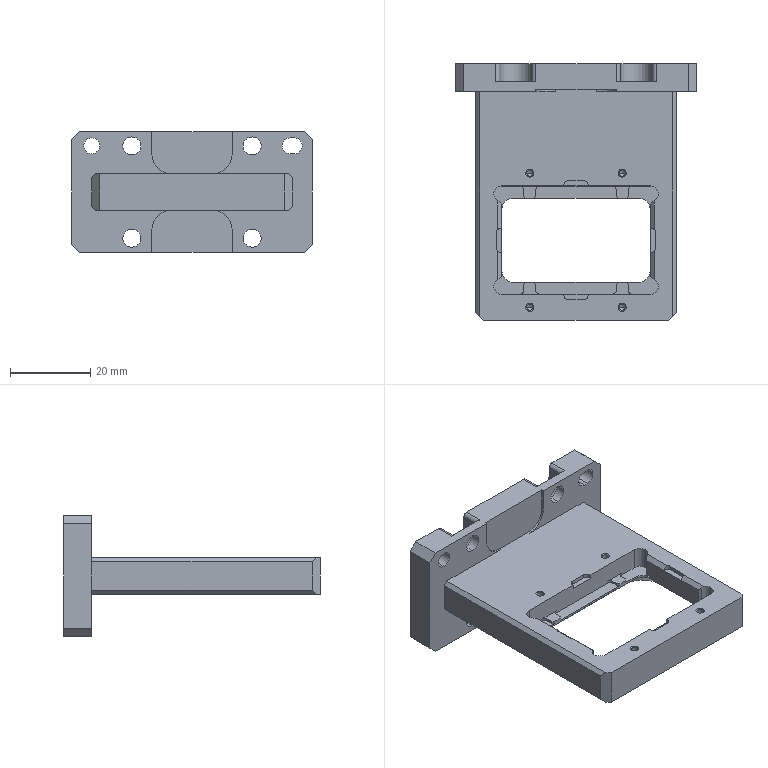NC program | NX | posted with a generic post | part box 60 x 64 x 30 mm
Lines 1 to 592 of 2202:
N10 G17 G21 G94 G90
(ZLEVEL_PROFILE_1 , TOOL : D6)
N12 T06 M6
N14 G54
N16 G17 G0 G90 X20.505 Y-18.6 B0. C0. S9500 M3
N18 G43 Z30. H6
N20 Z0.54
N22 G94 G1 Z-0.46 F1650.
N24 X20.356 Y-18.317
N26 G3 X19.848 Y-17.997 R0.6
N28 G2 X16. Y-14. R4.
N30 G1 Y-11.48
N32 G3 X15. Y-10.48 R1.
N34 X14. Y-11.48 R1.
N36 G1 Y-14.
N38 G2 X10.159 Y-17.997 R4.
N40 G3 X9.652 Y-18.317 R0.6
N42 G1 X9.503 Y-18.6
N44 Z0.54
N46 G0 X20.507 Z0.08
N48 G1 Z-0.92
N50 X20.356 Y-18.316
N52 G3 X19.848 Y-17.997 R0.6
N54 G1 X19.823 Y-17.996
N56 G2 X16. Y-14. R4.
N58 G1 Y-11.48
N60 G3 X15. Y-10.48 R1.
N62 X14. Y-11.48 R1.
N64 G1 Y-14.
N66 G2 X10.159 Y-17.996 R4.
N68 G3 X9.646 Y-18.308 R0.6
N70 G1 X9.487 Y-18.6
N72 Z0.08
N74 G0 X20.483 Z-0.38
N76 G1 Z-1.38
N78 X20.345 Y-18.326
N80 G3 X19.843 Y-17.997 R0.6
N82 G1 X19.823 Y-17.996
N84 G2 X16. Y-14. R4.
N86 G1 Y-11.48
N88 G3 X15. Y-10.48 R1.
N90 X14. Y-11.48 R1.
N92 G1 Y-14.
N94 G2 X10.159 Y-17.997 R4.
N96 G3 X9.649 Y-18.312 R0.6
N98 G1 X9.494 Y-18.6
N100 Z-0.38
N102 G0 X20.467 Z-0.84
N104 G1 Z-1.84
N106 X20.339 Y-18.335
N108 G3 X19.843 Y-17.998 R0.6
N110 G1 X19.823 Y-17.996
N112 G2 X16. Y-14. R4.
N114 G1 Y-11.48
N116 G3 X15. Y-10.48 R1.
N118 X14. Y-11.48 R1.
N120 G1 Y-14.
N122 G2 X10.159 Y-17.997 R4.
N124 G3 X9.651 Y-18.316 R0.6
N126 G1 X9.501 Y-18.6
N128 Z-0.84
N130 G0 X20.451 Z-1.3
N132 G1 Z-2.3
N134 X20.333 Y-18.344
N136 G3 X19.843 Y-17.998 R0.6
N138 G1 X19.823 Y-17.996
N140 G2 X16. Y-14. R4.
N142 G1 Y-11.48
N144 G3 X15. Y-10.48 R1.
N146 X14. Y-11.48 R1.
N148 G1 Y-14.
N150 G2 X10.159 Y-17.997 R4.
N152 G3 X9.654 Y-18.32 R0.6
N154 G1 X9.509 Y-18.6
N156 Z-1.3
N158 G0 X20.436 Z-1.76
N160 G1 Z-2.76
N162 X20.327 Y-18.353
N164 G3 X19.843 Y-17.998 R0.6
N166 G1 X19.823 Y-17.996
N168 G2 X16. Y-14. R4.
N170 G1 Y-11.48
N172 G3 X15. Y-10.48 R1.
N174 X14. Y-11.48 R1.
N176 G1 Y-14.
N178 G2 X10.159 Y-17.997 R4.
N180 G3 X9.656 Y-18.324 R0.6
N182 G1 X9.516 Y-18.6
N184 Z-1.76
N186 G0 X20.421 Z-2.22
N188 G1 Z-3.22
N190 X20.321 Y-18.361
N192 G3 X19.843 Y-17.999 R0.6
N194 G1 X19.823 Y-17.996
N196 G2 X16. Y-14. R4.
N198 G1 Y-11.48
N200 G3 X15. Y-10.48 R1.
N202 X14. Y-11.48 R1.
N204 G1 Y-14.
N206 G2 X10.159 Y-17.997 R4.
N208 G3 X9.659 Y-18.328 R0.6
N210 G1 X9.523 Y-18.6
N212 Z-2.22
N214 G0 X20.406 Z-2.68
N216 G1 Z-3.68
N218 X20.314 Y-18.37
N220 G3 X19.843 Y-17.999 R0.6
N222 G1 X19.823 Y-17.996
N224 G2 X16. Y-14. R4.
N226 G1 Y-11.48
N228 G3 X15. Y-10.48 R1.
N230 X14. Y-11.48 R1.
N232 G1 Y-14.
N234 G2 X10.159 Y-17.997 R4.001
N236 G3 X9.661 Y-18.332 R0.6
N238 G1 X9.53 Y-18.6
N240 Z-2.68
N242 G0 X20.392 Z-3.14
N244 G1 Z-4.14
N246 X20.308 Y-18.378
N248 G3 X19.843 Y-17.999 R0.6
N250 G1 X19.823 Y-17.996
N252 G2 X16. Y-14. R4.
N254 G1 Y-11.48
N256 G3 X15. Y-10.48 R1.
N258 X14. Y-11.48 R1.
N260 G1 Y-14.
N262 G2 X10.159 Y-17.997 R4.001
N264 G3 X9.664 Y-18.336 R0.6
N266 G1 X9.537 Y-18.6
N268 Z-3.14
N270 G0 X20.378 Z-3.6
N272 G1 Z-4.6
N274 X20.301 Y-18.387
N276 G3 X19.843 Y-18. R0.6
N278 G1 X19.823 Y-17.996
N280 G2 X16. Y-14. R4.
N282 G1 Y-11.48
N284 G3 X15. Y-10.48 R1.
N286 X14. Y-11.48 R1.
N288 G1 Y-14.
N290 G2 X10.159 Y-17.998 R4.001
N292 G3 X9.666 Y-18.34 R0.6
N294 G1 X9.543 Y-18.6
N296 Z-3.6
N298 G0 Z30.
N300 X9.483 Y18.6
N302 Z0.54
N304 G1 Z-0.46
N306 X9.634 Y18.316
N308 G3 X10.143 Y17.997 R0.6
N310 G2 X14. Y14. R4.
N312 G1 Y11.52
N314 G3 X15. Y10.52 R1.
N316 X16. Y11.52 R1.
N318 G1 Y14.
N320 G2 X19.831 Y17.996 R4.
N322 G1 X19.866 Y17.997
N324 G3 X20.378 Y18.309 R0.6
N326 G1 X20.538 Y18.6
N328 Z0.54
N330 G0 X9.483 Z0.08
N332 G1 Z-0.92
N334 X9.634 Y18.316
N336 G3 X10.143 Y17.997 R0.6
N338 G2 X14. Y14. R4.
N340 G1 Y11.52
N342 G3 X15. Y10.52 R1.
N344 X16. Y11.52 R1.
N346 G1 Y14.
N348 G2 X19.831 Y17.996 R4.
N350 G1 X19.861 Y17.997
N352 G3 X20.371 Y18.314 R0.6
N354 G1 X20.524 Y18.6
N356 Z0.08
N358 G0 X9.474 Z-0.38
N360 G1 Z-1.38
N362 X9.631 Y18.311
N364 G3 X10.143 Y17.997 R0.6
N366 G1 X10.163
N368 G2 X14. Y14. R4.
N370 G1 Y11.52
N372 G3 X15. Y10.52 R1.
N374 X16. Y11.52 R1.
N376 G1 Y14.
N378 G2 X19.831 Y17.996 R4.
N380 G1 X19.861 Y17.998
N382 G3 X20.367 Y18.319 R0.6
N384 G1 X20.514 Y18.6
N386 Z-0.38
N388 G0 X9.481 Z-0.84
N390 G1 Z-1.84
N392 X9.633 Y18.315
N394 G3 X10.143 Y17.997 R0.6
N396 G1 X10.163
N398 G2 X14. Y14. R4.
N400 G1 Y11.52
N402 G3 X15. Y10.52 R1.
N404 X16. Y11.52 R1.
N406 G1 Y14.
N408 G2 X19.831 Y17.996 R4.
N410 G1 X19.861 Y17.998
N412 G3 X20.364 Y18.324 R0.6
N414 G1 X20.505 Y18.6
N416 Z-0.84
N418 G0 X9.488 Z-1.3
N420 G1 Z-2.3
N422 X9.636 Y18.319
N424 G3 X10.143 Y17.998 R0.6
N426 G1 X10.163 Y17.997
N428 G2 X14. Y14. R4.
N430 G1 Y11.52
N432 G3 X15. Y10.52 R1.
N434 X16. Y11.52 R1.
N436 G1 Y14.
N438 G2 X19.831 Y17.996 R4.
N440 G1 X19.861 Y17.998
N442 G3 X20.361 Y18.33 R0.6
N444 G1 X20.495 Y18.6
N446 Z-1.3
N448 G0 X9.496 Z-1.76
N450 G1 Z-2.76
N452 X9.638 Y18.323
N454 G3 X10.143 Y17.998 R0.6
N456 G1 X10.163 Y17.997
N458 G2 X14. Y14. R4.
N460 G1 Y11.52
N462 G3 X15. Y10.52 R1.
N464 X16. Y11.52 R1.
N466 G1 Y14.
N468 G2 X19.831 Y17.996 R4.
N470 G1 X19.861 Y17.999
N472 G3 X20.358 Y18.335 R0.6
N474 G1 X20.486 Y18.6
N476 Z-1.76
N478 G0 X9.503 Z-2.22
N480 G1 Z-3.22
N482 X9.641 Y18.327
N484 G3 X10.143 Y17.998 R0.6
N486 G1 X10.163 Y17.997
N488 G2 X14. Y14. R4.
N490 G1 Y11.52
N492 G3 X15. Y10.52 R1.
N494 X16. Y11.52 R1.
N496 G1 Y14.
N498 G2 X19.831 Y17.996 R4.
N500 G1 X19.861 Y17.999
N502 G3 X20.354 Y18.34 R0.6
N504 G1 X20.477 Y18.6
N506 Z-2.22
N508 G0 X9.51 Z-2.68
N510 G1 Z-3.68
N512 X9.643 Y18.33
N514 G3 X10.143 Y17.998 R0.6
N516 G1 X10.163 Y17.997
N518 G2 X14. Y14. R4.
N520 G1 Y11.52
N522 G3 X15. Y10.52 R1.
N524 X16. Y11.52 R1.
N526 G1 Y14.
N528 G2 X19.831 Y17.996 R4.
N530 G1 X19.861 Y17.999
N532 G3 X20.351 Y18.345 R0.6
N534 G1 X20.468 Y18.6
N536 Z-2.68
N538 G0 X9.516 Z-3.14
N540 G1 Z-4.14
N542 X9.646 Y18.334
N544 G3 X10.143 Y17.998 R0.6
N546 G1 X10.163 Y17.997
N548 G2 X14. Y14. R4.
N550 G1 Y11.52
N552 G3 X15. Y10.52 R1.
N554 X16. Y11.52 R1.
N556 G1 Y14.
N558 G2 X19.831 Y17.996 R4.
N560 G1 X19.861 Y17.999
N562 G3 X20.347 Y18.35 R0.6
N564 G1 X20.46 Y18.6
N566 Z-3.14
N568 G0 X9.523 Z-3.6
N570 G1 Z-4.6
N572 X9.648 Y18.338
N574 G3 X10.143 Y17.998 R0.6
N576 G1 X10.163 Y17.997
N578 G2 X14. Y14. R4.
N580 G1 Y11.52
N582 G3 X15. Y10.52 R1.
N584 X16. Y11.52 R1.
N586 G1 Y14.
N588 G2 X19.831 Y17.996 R4.
N590 G1 X19.861 Y18.
N592 G3 X20.344 Y18.355 R0.6
N594 G1 X20.451 Y18.6
N596 Z-3.6
N598 G0 Z30.
N600 X-20.517
N602 Z0.54
N604 G1 Z-0.46
N606 X-20.366 Y18.316
N608 G3 X-19.857 Y17.997 R0.6
N610 G2 X-16. Y14. R4.
N612 G1 Y11.52
N614 G3 X-15. Y10.52 R1.
N616 X-14. Y11.52 R1.
N618 G1 Y14.
N620 G2 X-10.169 Y17.996 R4.
N622 G1 X-10.134 Y17.997
N624 G3 X-9.622 Y18.309 R0.6
N626 G1 X-9.462 Y18.6
N628 Z0.54
N630 G0 X-20.517 Z0.08
N632 G1 Z-0.92
N634 X-20.366 Y18.316
N636 G3 X-19.857 Y17.997 R0.6
N638 G2 X-16. Y14. R4.
N640 G1 Y11.52
N642 G3 X-15. Y10.52 R1.
N644 X-14. Y11.52 R1.
N646 G1 Y14.
N648 G2 X-10.169 Y17.996 R4.
N650 G1 X-10.139 Y17.997
N652 G3 X-9.629 Y18.314 R0.6
N654 G1 X-9.476 Y18.6
N656 Z0.08
N658 G0 X-20.526 Z-0.38
N660 G1 Z-1.38
N662 X-20.369 Y18.311
N664 G3 X-19.857 Y17.997 R0.6
N666 G1 X-19.837
N668 G2 X-16. Y14. R4.
N670 G1 Y11.52
N672 G3 X-15. Y10.52 R1.
N674 X-14. Y11.52 R1.
N676 G1 Y14.
N678 G2 X-10.169 Y17.996 R4.
N680 G1 X-10.139 Y17.998
N682 G3 X-9.633 Y18.319 R0.6
N684 G1 X-9.486 Y18.6
N686 Z-0.38
N688 G0 X-20.519 Z-0.84
N690 G1 Z-1.84
N692 X-20.367 Y18.315
N694 G3 X-19.857 Y17.997 R0.6
N696 G1 X-19.837
N698 G2 X-16. Y14. R4.
N700 G1 Y11.52
N702 G3 X-15. Y10.52 R1.
N704 X-14. Y11.52 R1.
N706 G1 Y14.
N708 G2 X-10.169 Y17.996 R4.
N710 G1 X-10.139 Y17.998
N712 G3 X-9.636 Y18.324 R0.6
N714 G1 X-9.495 Y18.6
N716 Z-0.84
N718 G0 X-20.512 Z-1.3
N720 G1 Z-2.3
N722 X-20.364 Y18.319
N724 G3 X-19.857 Y17.998 R0.6
N726 G1 X-19.837 Y17.997
N728 G2 X-16. Y14. R4.
N730 G1 Y11.52
N732 G3 X-15. Y10.52 R1.
N734 X-14. Y11.52 R1.
N736 G1 Y14.
N738 G2 X-10.169 Y17.996 R4.
N740 G1 X-10.139 Y17.998
N742 G3 X-9.639 Y18.33 R0.6
N744 G1 X-9.505 Y18.6
N746 Z-1.3
N748 G0 X-20.504 Z-1.76
N750 G1 Z-2.76
N752 X-20.362 Y18.323
N754 G3 X-19.857 Y17.998 R0.6
N756 G1 X-19.837 Y17.997
N758 G2 X-16. Y14. R4.
N760 G1 Y11.52
N762 G3 X-15. Y10.52 R1.
N764 X-14. Y11.52 R1.
N766 G1 Y14.
N768 G2 X-10.169 Y17.996 R4.
N770 G1 X-10.139 Y17.999
N772 G3 X-9.642 Y18.335 R0.6
N774 G1 X-9.514 Y18.6
N776 Z-1.76
N778 G0 X-20.497 Z-2.22
N780 G1 Z-3.22
N782 X-20.359 Y18.327
N784 G3 X-19.857 Y17.998 R0.6
N786 G1 X-19.837 Y17.997
N788 G2 X-16. Y14. R4.
N790 G1 Y11.52
N792 G3 X-15. Y10.52 R1.
N794 X-14. Y11.52 R1.
N796 G1 Y14.
N798 G2 X-10.169 Y17.996 R4.
N800 G1 X-10.139 Y17.999
N802 G3 X-9.646 Y18.34 R0.6
N804 G1 X-9.523 Y18.6
N806 Z-2.22
N808 G0 X-20.49 Z-2.68
N810 G1 Z-3.68
N812 X-20.357 Y18.33
N814 G3 X-19.857 Y17.998 R0.6
N816 G1 X-19.837 Y17.997
N818 G2 X-16. Y14. R4.
N820 G1 Y11.52
N822 G3 X-15. Y10.52 R1.
N824 X-14. Y11.52 R1.
N826 G1 Y14.
N828 G2 X-10.169 Y17.996 R4.
N830 G1 X-10.139 Y17.999
N832 G3 X-9.649 Y18.345 R0.6
N834 G1 X-9.532 Y18.6
N836 Z-2.68
N838 G0 X-20.484 Z-3.14
N840 G1 Z-4.14
N842 X-20.354 Y18.334
N844 G3 X-19.857 Y17.998 R0.6
N846 G1 X-19.837 Y17.997
N848 G2 X-16. Y14. R4.
N850 G1 Y11.52
N852 G3 X-15. Y10.52 R1.
N854 X-14. Y11.52 R1.
N856 G1 Y14.
N858 G2 X-10.169 Y17.996 R4.
N860 G1 X-10.139 Y17.999
N862 G3 X-9.653 Y18.35 R0.6
N864 G1 X-9.54 Y18.6
N866 Z-3.14
N868 G0 X-20.477 Z-3.6
N870 G1 Z-4.6
N872 X-20.352 Y18.338
N874 G3 X-19.857 Y17.998 R0.6
N876 G1 X-19.837 Y17.997
N878 G2 X-16. Y14. R4.
N880 G1 Y11.52
N882 G3 X-15. Y10.52 R1.
N884 X-14. Y11.52 R1.
N886 G1 Y14.
N888 G2 X-10.169 Y17.996 R4.
N890 G1 X-10.139 Y18.
N892 G3 X-9.656 Y18.355 R0.6
N894 G1 X-9.549 Y18.6
N896 Z-3.6
N898 G0 Z30.
N900 X-9.495 Y-18.6
N902 Z0.54
N904 G1 Z-0.46
N906 X-9.644 Y-18.317
N908 G3 X-10.152 Y-17.997 R0.6
N910 G2 X-14. Y-14. R4.
N912 G1 Y-11.48
N914 G3 X-15. Y-10.48 R1.
N916 X-16. Y-11.48 R1.
N918 G1 Y-14.
N920 G2 X-19.841 Y-17.997 R4.
N922 G3 X-20.348 Y-18.317 R0.6
N924 G1 X-20.497 Y-18.6
N926 Z0.54
N928 G0 X-9.493 Z0.08
N930 G1 Z-0.92
N932 X-9.644 Y-18.316
N934 G3 X-10.152 Y-17.997 R0.6
N936 G1 X-10.177 Y-17.996
N938 G2 X-14. Y-14. R4.
N940 G1 Y-11.48
N942 G3 X-15. Y-10.48 R1.
N944 X-16. Y-11.48 R1.
N946 G1 Y-14.
N948 G2 X-19.841 Y-17.996 R4.
N950 G3 X-20.354 Y-18.308 R0.6
N952 G1 X-20.513 Y-18.6
N954 Z0.08
N956 G0 X-9.517 Z-0.38
N958 G1 Z-1.38
N960 X-9.655 Y-18.326
N962 G3 X-10.157 Y-17.997 R0.6
N964 G1 X-10.177 Y-17.996
N966 G2 X-14. Y-14. R4.
N968 G1 Y-11.48
N970 G3 X-15. Y-10.48 R1.
N972 X-16. Y-11.48 R1.
N974 G1 Y-14.
N976 G2 X-19.841 Y-17.997 R4.
N978 G3 X-20.351 Y-18.312 R0.6
N980 G1 X-20.506 Y-18.6
N982 Z-0.38
N984 G0 X-9.533 Z-0.84
N986 G1 Z-1.84
N988 X-9.661 Y-18.335
N990 G3 X-10.157 Y-17.998 R0.6
N992 G1 X-10.177 Y-17.996
N994 G2 X-14. Y-14. R4.
N996 G1 Y-11.48
N998 G3 X-15. Y-10.48 R1.
N1000 X-16. Y-11.48 R1.
N1002 G1 Y-14.
N1004 G2 X-19.841 Y-17.997 R4.
N1006 G3 X-20.349 Y-18.316 R0.6
N1008 G1 X-20.499 Y-18.6
N1010 Z-0.84
N1012 G0 X-9.549 Z-1.3
N1014 G1 Z-2.3
N1016 X-9.667 Y-18.344
N1018 G3 X-10.157 Y-17.998 R0.6
N1020 G1 X-10.177 Y-17.996
N1022 G2 X-14. Y-14. R4.
N1024 G1 Y-11.48
N1026 G3 X-15. Y-10.48 R1.
N1028 X-16. Y-11.48 R1.
N1030 G1 Y-14.
N1032 G2 X-19.841 Y-17.997 R4.
N1034 G3 X-20.346 Y-18.32 R0.6
N1036 G1 X-20.491 Y-18.6
N1038 Z-1.3
N1040 G0 X-9.564 Z-1.76
N1042 G1 Z-2.76
N1044 X-9.673 Y-18.353
N1046 G3 X-10.157 Y-17.998 R0.6
N1048 G1 X-10.177 Y-17.996
N1050 G2 X-14. Y-14. R4.
N1052 G1 Y-11.48
N1054 G3 X-15. Y-10.48 R1.
N1056 X-16. Y-11.48 R1.
N1058 G1 Y-14.
N1060 G2 X-19.841 Y-17.997 R4.
N1062 G3 X-20.344 Y-18.324 R0.6
N1064 G1 X-20.484 Y-18.6
N1066 Z-1.76
N1068 G0 X-9.579 Z-2.22
N1070 G1 Z-3.22
N1072 X-9.679 Y-18.361
N1074 G3 X-10.157 Y-17.999 R0.6
N1076 G1 X-10.177 Y-17.996
N1078 G2 X-14. Y-14. R4.
N1080 G1 Y-11.48
N1082 G3 X-15. Y-10.48 R1.
N1084 X-16. Y-11.48 R1.
N1086 G1 Y-14.
N1088 G2 X-19.841 Y-17.997 R4.
N1090 G3 X-20.341 Y-18.328 R0.6
N1092 G1 X-20.477 Y-18.6
N1094 Z-2.22
N1096 G0 X-9.594 Z-2.68
N1098 G1 Z-3.68
N1100 X-9.686 Y-18.37
N1102 G3 X-10.157 Y-17.999 R0.6
N1104 G1 X-10.177 Y-17.996
N1106 G2 X-14. Y-14. R4.
N1108 G1 Y-11.48
N1110 G3 X-15. Y-10.48 R1.
N1112 X-16. Y-11.48 R1.
N1114 G1 Y-14.
N1116 G2 X-19.841 Y-17.997 R4.001
N1118 G3 X-20.339 Y-18.332 R0.6
N1120 G1 X-20.47 Y-18.6
N1122 Z-2.68
N1124 G0 X-9.608 Z-3.14
N1126 G1 Z-4.14
N1128 X-9.692 Y-18.378
N1130 G3 X-10.157 Y-17.999 R0.6
N1132 G1 X-10.177 Y-17.996
N1134 G2 X-14. Y-14. R4.
N1136 G1 Y-11.48
N1138 G3 X-15. Y-10.48 R1.
N1140 X-16. Y-11.48 R1.
N1142 G1 Y-14.
N1144 G2 X-19.841 Y-17.997 R4.001
N1146 G3 X-20.336 Y-18.336 R0.6
N1148 G1 X-20.463 Y-18.6
N1150 Z-3.14
N1152 G0 X-9.622 Z-3.6
N1154 G1 Z-4.6
N1156 X-9.699 Y-18.387
N1158 G3 X-10.157 Y-18. R0.6
N1160 G1 X-10.177 Y-17.996
N1162 G2 X-14. Y-14. R4.
N1164 G1 Y-11.48
N1166 G3 X-15. Y-10.48 R1.
N1168 X-16. Y-11.48 R1.
N1170 G1 Y-14.
N1172 G2 X-19.841 Y-17.998 R4.001
N1174 G3 X-20.334 Y-18.34 R0.6
N1176 G1 X-20.457 Y-18.6
N1178 Z-3.6
N1180 G0 Z30.
N1182 M5